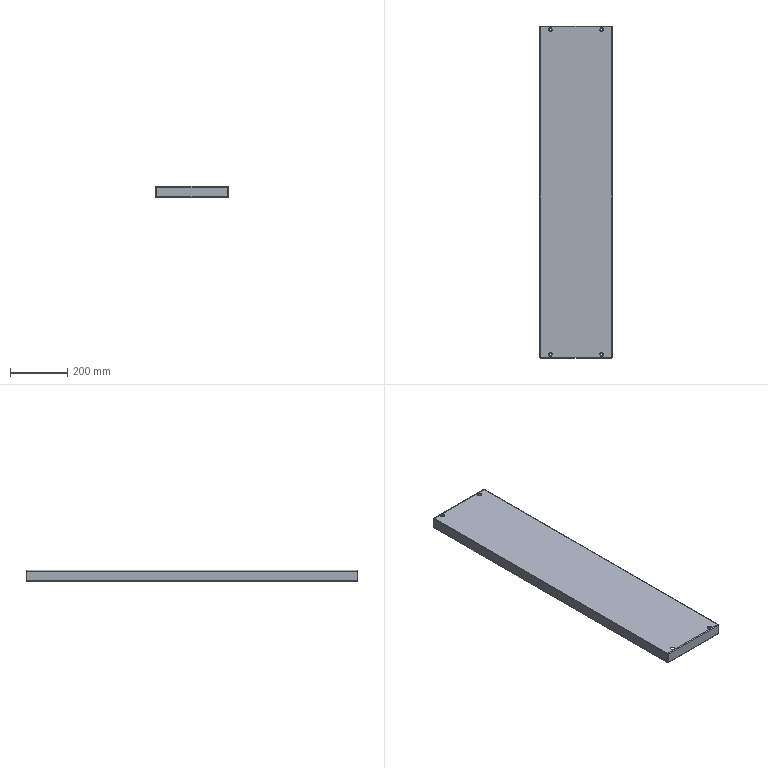Part | STEP file | SX-020-01 | 1 solid | 86 faces | box 251.001 x 1156 x 39 mm | volume 904876 mm3 | plane 42 | cylinder 32 | spline 12 | commonest cylinder face diameters 0.4 x8 4.4 x8 8 x8 14 x8